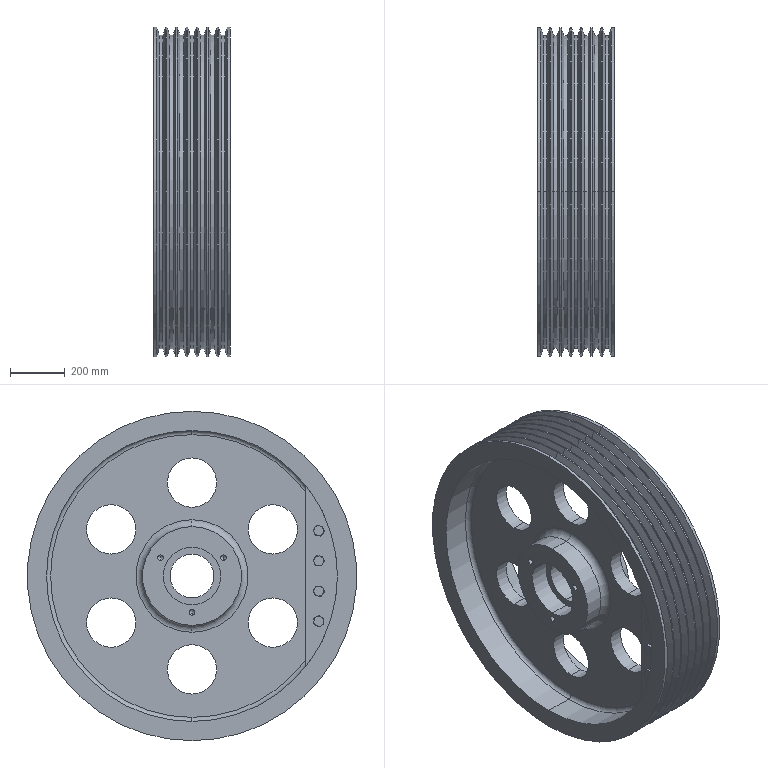Part | SolidWorks | features CompositeCurve 1 | 15 solids | 347 faces | box 280 x 1200 x 1200 mm | volume 105552059 mm3 | cylinder 142 | plane 97 | cone 92 | torus 16 | commonest cylinder face diameters 25 x24 1200 x16 1143 x14 24.5 x12 36.439 x12 180 x12